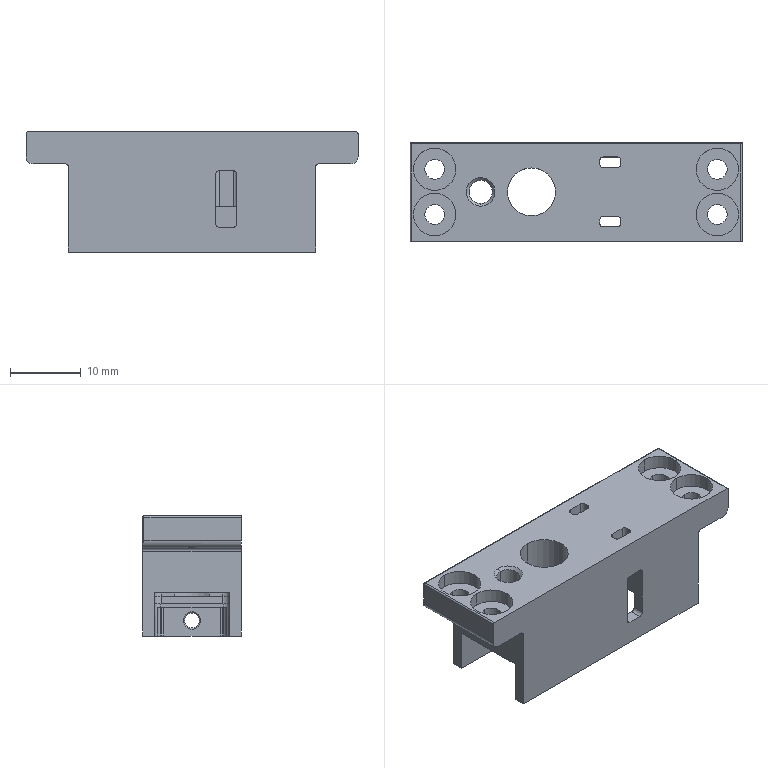NC program | NX | posted with a generic post | part box 47 x 14 x 17 mm
Lines 1 to 364 of 2938:
N10 G17 G21 G94 G90
(FLOOR_WALL , TOOL : D63)
N12 T01 M6
N14 G54
N16 G17 G0 G90 X-61. Y0. B0. C0. S6500 M3
N18 G43 Z30. H1
N20 Z3.
N22 G94 G1 Z0. F1250.
N24 X-58.
N26 X58.
N28 X61.
N30 Z3.
N32 G0 Z30.
N34 M5
(DRILLING_COPY_1 , TOOL : D6A45)
N36 T18 M6
N38 G54
N40 G17 G0 G90 X20. Y3.2 B0. C0. S3000 M3
N42 G43 Z30. H18
N44 G94 G81 G98 Z-1. F200. R3.
N46 Y-3.2
N48 X-6.3 Y0.
N50 X-13.5
N52 X-20. Y3.2
N54 Y-3.2
N56 G80
N58 G0 X-20. Y-3.2 Z30.
N60 M5
(DRILLING_COPY_1_COPY , TOOL : 3.4ZT)
N62 T13 M6
N64 G54
N66 G17 G0 G90 X-13.5 Y0. B0. C0. S2000 M3
N68 G43 Z30. H13
N70 G94 G83 G98 Z-13.391 F150. Q2. R3.
N72 G80
N74 G0 X-13.5 Y0. Z30.
N76 M5
(DRILLING_COPY_1_COPY_COPY_1 , TOOL : 2.8ZT)
N78 T17 M6
N80 G54
N82 G17 G0 G90 X-20. Y3.2 B0. C0. S2000 M3
N84 G43 Z30. H17
N86 G94 G83 G98 Z-6.841 F150. Q2. R3.
N88 Y-3.2
N90 X20.
N92 Y3.2
N94 G80
N96 G0 X20. Y3.2 Z30.
N98 M5
(DRILLING_COPY_1_COPY_COPY_1_COPY , TOOL : 7.0ZT)
N100 T12 M6
N102 G54
N104 G17 G0 G90 X-6.3 Y0. B0. C0. S2000 M3
N106 G43 Z30. H12
N108 G94 G83 G98 Z-8.943 F300. Q2. R3.
N110 G80
N112 G0 X-6.3 Y0. Z30.
N114 M5
(ADAPTIVE_MILLING , TOOL : D10)
N116 T03 M6
N118 G54
N120 G17 G0 G90 X-34.136 Y-0.037 B0. C0. S8000 M3
N122 G43 Z30. H3
N124 Z-14.
N126 G94 G1 Z-17. F1000.
N128 X-31.974 Y-0.361 F3500.
N130 G3 X-31.511 Y-0.037 R0.512
N132 X-31.007 Y3.469 R12.033
N134 G2 X-30.874 Y8.265 R171.805
N136 X-27.693 Y12.587 R6.204
N138 X-22.178 Y14.141 R13.475
N140 X-12.735 Y14.388 R113.004
N142 G1 X-9.885 Y14.392
N144 X-1.785 Y14.393
N146 X24.165
N148 X24.24 Y14.391
N150 X24.39 Y14.384
N152 X24.54 Y14.372
N154 G2 X29.009 Y11.294 R6.094
N156 X30.626 Y5.8 R13.086
N158 X30.884 Y-2.743 R96.287
N160 X30.852 Y-8.216 R106.001
N162 X27.709 Y-12.562 R6.156
N164 X22.2 Y-14.137 R13.359
N166 X14.032 Y-14.385 R95.055
N168 G1 X12.007 Y-14.39
N170 X8.407 Y-14.392
N172 X-16.943 Y-14.393
N174 X-24.143
N176 X-24.293 Y-14.39
N178 X-24.368 Y-14.386
N180 G2 X-28.918 Y-11.44 R6.007
N182 X-30.615 Y-5.896 R12.746
N184 X-30.638 Y0.241 R27.34
N186 G3 X-30.316 Y6.156 R854.514
N188 G2 X-25.942 Y11.973 R7.781
N190 X-19.726 Y13.533 R16.704
N192 X-10.057 Y13.78 R128.639
N194 G1 X-7.507 Y13.784
N196 X-2.332 Y13.786
N198 X21.743 Y13.787
N200 X21.893 Y13.785
N202 X22.043 Y13.78
N204 X22.193 Y13.772
N206 G2 X28.293 Y9.714 R7.569
N208 X30. Y3.542 R15.66
N210 X30.232 Y-6.049 R85.193
N212 X26.091 Y-11.858 R7.63
N214 X19.903 Y-13.514 R15.985
N216 X9.635 Y-13.781 R126.768
N218 G1 X6.935 Y-13.785
N220 X0.785 Y-13.786
N222 X-21.715 Y-13.787
N224 X-21.865 Y-13.785
N226 X-22.015 Y-13.781
N228 X-22.165 Y-13.774
N230 G2 X-28.28 Y-9.74 R7.556
N232 X-29.995 Y-2.516 R15.193
N234 X-29.73 Y4.675 R76.659
N236 X-28.483 Y8.067 R9.926
N238 X-27.055 Y10.604 R5.904
N240 X-23.921 Y12.15 R6.23
N242 X-14.913 Y13.102 R44.286
N244 X-2.688 Y13.179 R678.947
N246 G1 X11.337 Y13.18
N248 X19.662
N250 X19.887 Y13.178
N252 X20.112 Y13.173
N254 X20.336 Y13.164
N256 X20.486 Y13.156
N258 G2 X24.277 Y12.048 R8.793
N260 G1 X24.798 Y11.979
N262 X24.865 Y11.961
N264 G2 X27.163 Y10.614 R5.904
N266 X28.678 Y7.42 R6.
N268 X29.617 Y-2.192 R48.847
N270 X29.034 Y-6.692 R10.639
N272 G1 X28.976 Y-6.83
N274 X28.916 Y-6.968
N276 X28.854 Y-7.104
N278 X28.788 Y-7.239
N280 X28.721 Y-7.373
N282 X28.651 Y-7.506
N284 X28.615 Y-7.571
N286 X28.582 Y-7.639
N288 X28.555 Y-7.721
N290 X28.479 Y-8.298
N292 X28.461 Y-8.365
N294 G2 X27.114 Y-10.663 R5.904
N296 X23.847 Y-12.195 R6.062
N298 X14.158 Y-13.12 R49.02
N300 X1.258 Y-13.18 R720.573
N302 G1 X-19.667
N304 X-19.892 Y-13.178
N306 X-20.117 Y-13.173
N308 X-20.342 Y-13.164
N310 X-20.491 Y-13.156
N312 G2 X-24.277 Y-12.048 R8.827
N314 G1 X-24.798 Y-11.979
N316 X-24.865 Y-11.961
N318 G2 X-27.163 Y-10.614 R5.904
N320 X-28.708 Y-7.273 R6.097
N322 X-29.286 Y0.712 R34.298
N324 X-28.65 Y5.411 R14.972
N326 X-28.481 Y8.082 R12.304
N328 G1 X-28.454 Y8.217
N330 X-28.19 Y8.863
N332 X-27.912 Y9.503
N334 X-27.49 Y10.059
N336 X-27.055 Y10.604
N338 X-26.504 Y11.032
N340 X-25.942 Y11.447
N342 X-25.299 Y11.717
N344 X-24.65 Y11.972
N346 G2 X-21.783 Y12.163 R14.936
N348 X-4.091 Y12.571 R263.395
N350 G1 X0.934 Y12.573
N352 X17.884
N354 X18.184 Y12.57
N356 X18.484 Y12.564
N358 X18.634 Y12.56
N360 G2 X21.425 Y12.15 R14.25
N362 X24.335 Y12.04 R16.021
N364 G3 X24.409 Y13.135 R-0.55
N366 G1 X-22.322 Y13.243
N368 G3 X-22.232 Y12.15 R0.55
N370 G1 X21.493
N372 X23.517 Y12.148
N374 X24.193 Y12.062
N376 X24.865 Y11.961
N378 X25.487 Y11.707
N380 X26.103 Y11.439
N382 X26.638 Y11.032
N384 X27.163 Y10.614
N386 X27.574 Y10.083
N388 X27.974 Y9.542
N390 X28.234 Y8.923
N392 X28.479 Y8.298
N394 G2 X28.671 Y5.183 R18.169
N396 X28.957 Y-2.61 R103.627
N398 X28.65 Y-4.702 R17.647
N400 G1 Y-6.982
N402 X28.648 Y-7.017
N404 X28.55 Y-7.761
N406 G3 X29.645 Y-7.837 R-0.55
N408 G1 X29.743 Y5.944
N410 G3 X28.65 Y5.857 R0.55
N412 G1 Y-4.718
N414 X28.648 Y-7.017
N416 X28.562 Y-7.693
N418 X28.461 Y-8.365
N420 X28.207 Y-8.987
N422 X27.939 Y-9.603
N424 X27.532 Y-10.138
N426 X27.114 Y-10.663
N428 X26.583 Y-11.074
N430 X26.042 Y-11.474
N432 X25.423 Y-11.734
N434 X24.798 Y-11.979
N436 G2 X21.758 Y-12.167 R17.023
N438 X3.841 Y-12.571 R271.968
N440 G1 X-1.184 Y-12.573
N442 X-17.909
N444 X-18.209 Y-12.57
N446 X-18.434 Y-12.566
N448 X-18.659 Y-12.559
N450 X-18.734 Y-12.556
N452 G2 X-21.427 Y-12.15 R14.452
N454 X-24.335 Y-12.04 R16.002
N456 G3 X-24.409 Y-13.135 R-0.55
N458 G1 X22.447 Y-13.243
N460 G3 X22.357 Y-12.15 R0.55
N462 G1 X-21.443
N464 X-23.517 Y-12.148
N466 X-24.193 Y-12.062
N468 X-24.865 Y-11.961
N470 X-25.487 Y-11.707
N472 X-26.103 Y-11.439
N474 X-26.638 Y-11.032
N476 X-27.163 Y-10.614
N478 X-27.574 Y-10.083
N480 X-27.974 Y-9.542
N482 X-28.234 Y-8.923
N484 X-28.479 Y-8.298
N486 X-28.648 Y-7.017
N488 X-28.65 Y-6.982
N490 G2 X-28.65 Y5.47 R869.425
N492 G3 X-29.201 Y6.019 R0.55
N494 X-29.75 Y5.47 R0.55
N496 G1 X-29.742 Y-4.073
N498 G3 X-28.65 Y-3.982 R0.55
N500 G1 Y0.668
N502 G3 X-29.1 Y1.17 R0.509
N504 G1 X-31.083 Y1.389
N506 Z-14.
N508 G0 Z30.
N510 M5
(ZLEVEL_PROFILE_COPY , TOOL : D10JING)
N512 T07 M6
N514 G54
N516 G17 G0 G90 X25.122 Y-13.809 B0. C0. S8000 M3
N518 G43 Z30. H7
N520 Z-17.
N522 G94 G1 X24.366 Y-12.5 F1200.
N524 G3 X23.5 Y-12. R1.
N526 G1 X-23.5
N528 G2 X-28.5 Y-7. R5.
N530 G1 Y6.8
N532 G2 X-23.3 Y12. R5.2
N534 G1 X23.5
N536 G2 X28.5 Y7. R5.
N538 G1 Y-7.
N540 G2 X23.5 Y-12. R5.
N542 G3 X22.634 Y-12.5 R1.
N544 G1 X21.768 Y-14.
N546 G0 Z30.
N548 M5
(HOLE_MILLING , TOOL : D4)
N550 T10 M6
N552 G54
N554 G17 G0 G90 X-20. Y3.2 B0. C0. S9500 M3
N556 G43 Z30. H10
N558 Z0.5
N560 G94 G3 X-19.5 Y2.7 R0.5 F1300.
N562 X-19. Y3.2 R0.5
N564 X-19. Y3.2 Z0.1 I-1. J0.
N566 X-19. Y3.2 Z-0.3 I-1. J0.
N568 X-19. Y3.2 Z-0.7 I-1. J0.
N570 X-19. Y3.2 Z-1.1 I-1. J0.
N572 X-19. Y3.2 Z-1.5 I-1. J0.
N574 X-19. Y3.2 Z-1.9 I-1. J0.
N576 X-20. Y4.2 Z-2. R1.
N578 X-21. Y3.2 R1.
N580 X-20. Y4.2 R-1.
N582 X-20.5 Y3.7 R0.5
N584 X-20. Y3.2 R0.5
N586 G0 Z30.
N588 Y-3.2
N590 Z0.5
N592 G3 X-19.5 Y-3.7 R0.5
N594 X-19. Y-3.2 R0.5
N596 X-19. Y-3.2 Z0.1 I-1. J0.
N598 X-19. Y-3.2 Z-0.3 I-1. J0.
N600 X-19. Y-3.2 Z-0.7 I-1. J0.
N602 X-19. Y-3.2 Z-1.1 I-1. J0.
N604 X-19. Y-3.2 Z-1.5 I-1. J0.
N606 X-19. Y-3.2 Z-1.9 I-1. J0.
N608 X-20. Y-2.2 Z-2. R1.
N610 X-21. Y-3.2 R1.
N612 X-20. Y-2.2 R-1.
N614 X-20.5 Y-2.7 R0.5
N616 X-20. Y-3.2 R0.5
N618 G0 Z30.
N620 X20.
N622 Z0.5
N624 G3 X20.5 Y-3.7 R0.5
N626 X21. Y-3.2 R0.5
N628 X21. Y-3.2 Z0.1 I-1. J0.
N630 X21. Y-3.2 Z-0.3 I-1. J0.
N632 X21. Y-3.2 Z-0.7 I-1. J0.
N634 X21. Y-3.2 Z-1.1 I-1. J0.
N636 X21. Y-3.2 Z-1.5 I-1. J0.
N638 X21. Y-3.2 Z-1.9 I-1. J0.
N640 X20. Y-2.2 Z-2. R1.
N642 X19. Y-3.2 R1.
N644 X20. Y-2.2 R-1.
N646 X19.5 Y-2.7 R0.5
N648 X20. Y-3.2 R0.5
N650 G0 Z30.
N652 Y3.2
N654 Z0.5
N656 G3 X20.5 Y2.7 R0.5
N658 X21. Y3.2 R0.5
N660 X21. Y3.2 Z0.1 I-1. J0.
N662 X21. Y3.2 Z-0.3 I-1. J0.
N664 X21. Y3.2 Z-0.7 I-1. J0.
N666 X21. Y3.2 Z-1.1 I-1. J0.
N668 X21. Y3.2 Z-1.5 I-1. J0.
N670 X21. Y3.2 Z-1.9 I-1. J0.
N672 X20. Y4.2 Z-2. R1.
N674 X19. Y3.2 R1.
N676 X20. Y4.2 R-1.
N678 X19.5 Y3.7 R0.5
N680 X20. Y3.2 R0.5
N682 G0 Z30.
N684 M5